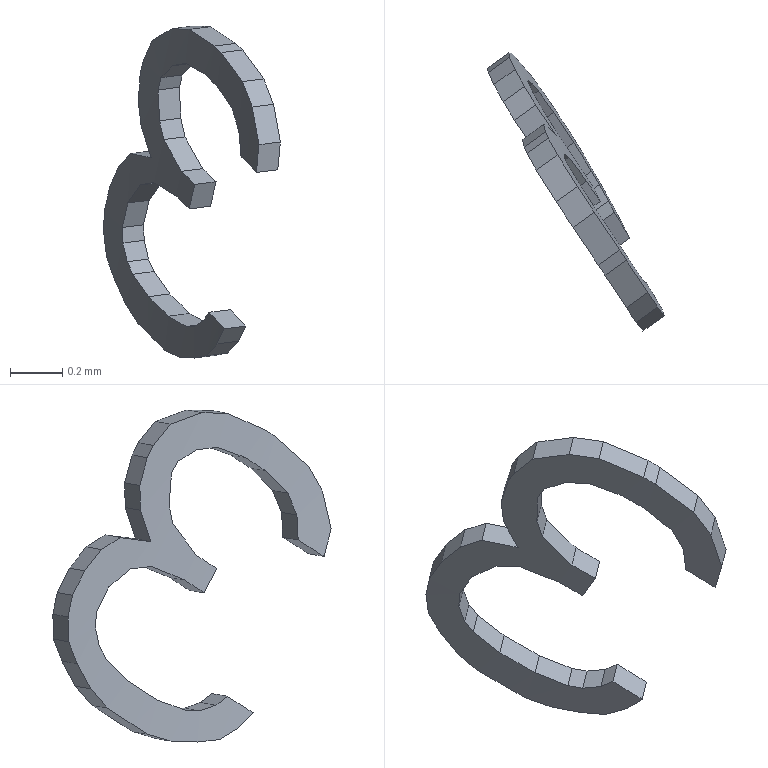Part | SolidWorks | features BaseBody 1 | 1 solid | 59 faces | box 0.6733 x 1.06 x 1.265 mm | volume 0.03834 mm3 | plane 57 | cylinder 2 | commonest cylinder face diameters 16.8 x1 17 x1